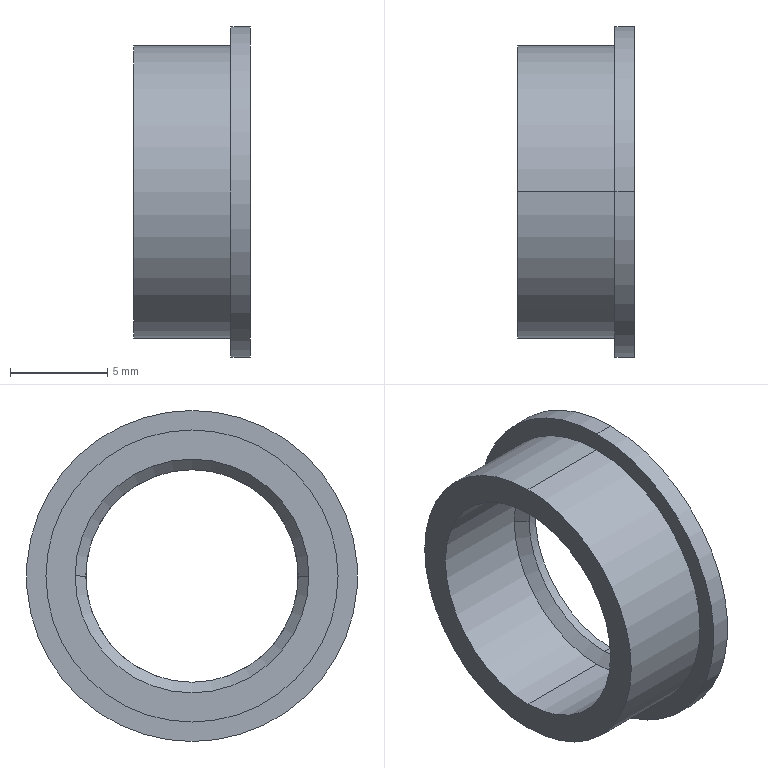Part | SolidWorks | features BaseBody 1 | 1 solid | 13 faces | box 6 x 17 x 17 mm | volume 446.259 mm3 | cylinder 8 | plane 3 | cone 2 | commonest cylinder face diameters 10.918 x2 12 x2 15 x2 17 x2
STEP:
#1=CARTESIAN_POINT('',(-6.5,0.,-7.5));
#2=VERTEX_POINT('',#1);
#3=CARTESIAN_POINT('',(-6.5,0.,7.5));
#4=VERTEX_POINT('',#3);
#5=CARTESIAN_POINT('',(-6.5,0.,0.));
#6=DIRECTION('',(1.,0.,0.));
#7=DIRECTION('',(0.,0.,-1.));
#8=AXIS2_PLACEMENT_3D('',#5,#6,#7);
#9=CIRCLE('',#8,7.5);
#10=EDGE_CURVE('',#2,#4,#9,.T.);
#11=ORIENTED_EDGE('',*,*,#10,.T.);
#12=CARTESIAN_POINT('',(-1.5,0.,7.5));
#13=VERTEX_POINT('',#12);
#14=CARTESIAN_POINT('',(-10.,0.,7.5));
#15=DIRECTION('',(1.,0.,0.));
#16=VECTOR('',#15,1000.);
#17=LINE('',#14,#16);
#18=EDGE_CURVE('',#4,#13,#17,.T.);
#19=ORIENTED_EDGE('',*,*,#18,.T.);
#20=CARTESIAN_POINT('',(-1.5,0.,-7.5));
#21=VERTEX_POINT('',#20);
#22=CARTESIAN_POINT('',(-1.5,0.,0.));
#23=DIRECTION('',(-1.,0.,0.));
#24=DIRECTION('',(0.,0.,-1.));
#25=AXIS2_PLACEMENT_3D('',#22,#23,#24);
#26=CIRCLE('',#25,7.5);
#27=EDGE_CURVE('',#13,#21,#26,.T.);
#28=ORIENTED_EDGE('',*,*,#27,.T.);
#29=CARTESIAN_POINT('',(-10.,0.,-7.5));
#30=DIRECTION('',(1.,0.,0.));
#31=VECTOR('',#30,1000.);
#32=LINE('',#29,#31);
#33=EDGE_CURVE('',#2,#21,#32,.T.);
#34=ORIENTED_EDGE('',*,*,#33,.F.);
#35=EDGE_LOOP('',(#11,#19,#28,#34));
#36=FACE_OUTER_BOUND('',#35,.T.);
#37=CARTESIAN_POINT('',(-10.,0.,0.));
#38=DIRECTION('',(1.,0.,0.));
#39=DIRECTION('',(0.,0.,-1.));
#40=AXIS2_PLACEMENT_3D('',#37,#38,#39);
#41=CYLINDRICAL_SURFACE('',#40,7.5);
#42=ADVANCED_FACE('',(#36),#41,.T.);
#43=CARTESIAN_POINT('',(-6.5,0.,6.));
#44=VERTEX_POINT('',#43);
#45=CARTESIAN_POINT('',(-6.5,0.,-6.));
#46=VERTEX_POINT('',#45);
#47=CARTESIAN_POINT('',(-6.5,0.,0.));
#48=DIRECTION('',(1.,0.,0.));
#49=DIRECTION('',(0.,0.,-1.));
#50=AXIS2_PLACEMENT_3D('',#47,#48,#49);
#51=CIRCLE('',#50,6.);
#52=EDGE_CURVE('',#44,#46,#51,.T.);
#53=ORIENTED_EDGE('',*,*,#52,.F.);
#54=CARTESIAN_POINT('',(-1.5,0.,6.));
#55=VERTEX_POINT('',#54);
#56=CARTESIAN_POINT('',(-10.,0.,6.));
#57=DIRECTION('',(1.,0.,0.));
#58=VECTOR('',#57,1000.);
#59=LINE('',#56,#58);
#60=EDGE_CURVE('',#44,#55,#59,.T.);
#61=ORIENTED_EDGE('',*,*,#60,.T.);
#62=CARTESIAN_POINT('',(-1.5,-6.,0.));
#63=VERTEX_POINT('',#62);
#64=CARTESIAN_POINT('',(-1.5,0.,0.));
#65=DIRECTION('',(-1.,0.,0.));
#66=DIRECTION('',(0.,0.,-1.));
#67=AXIS2_PLACEMENT_3D('',#64,#65,#66);
#68=CIRCLE('',#67,6.);
#69=EDGE_CURVE('',#63,#55,#68,.T.);
#70=ORIENTED_EDGE('',*,*,#69,.F.);
#71=CARTESIAN_POINT('',(-1.5,0.,-6.));
#72=VERTEX_POINT('',#71);
#73=CARTESIAN_POINT('',(-1.5,0.,0.));
#74=DIRECTION('',(-1.,0.,0.));
#75=DIRECTION('',(0.,0.,-1.));
#76=AXIS2_PLACEMENT_3D('',#73,#74,#75);
#77=CIRCLE('',#76,6.);
#78=EDGE_CURVE('',#72,#63,#77,.T.);
#79=ORIENTED_EDGE('',*,*,#78,.F.);
#80=CARTESIAN_POINT('',(-10.,0.,-6.));
#81=DIRECTION('',(1.,0.,0.));
#82=VECTOR('',#81,1000.);
#83=LINE('',#80,#82);
#84=EDGE_CURVE('',#46,#72,#83,.T.);
#85=ORIENTED_EDGE('',*,*,#84,.F.);
#86=EDGE_LOOP('',(#53,#61,#70,#79,#85));
#87=FACE_OUTER_BOUND('',#86,.T.);
#88=CARTESIAN_POINT('',(-10.,0.,0.));
#89=DIRECTION('',(1.,0.,0.));
#90=DIRECTION('',(0.,0.,-1.));
#91=AXIS2_PLACEMENT_3D('',#88,#89,#90);
#92=CYLINDRICAL_SURFACE('',#91,6.);
#93=ADVANCED_FACE('',(#87),#92,.F.);
#94=CARTESIAN_POINT('',(-1.5,0.,8.5));
#95=VERTEX_POINT('',#94);
#96=CARTESIAN_POINT('',(-1.5,0.,-8.5));
#97=VERTEX_POINT('',#96);
#98=CARTESIAN_POINT('',(-1.5,0.,0.));
#99=DIRECTION('',(-1.,0.,0.));
#100=DIRECTION('',(0.,0.,-1.));
#101=AXIS2_PLACEMENT_3D('',#98,#99,#100);
#102=CIRCLE('',#101,8.5);
#103=EDGE_CURVE('',#95,#97,#102,.T.);
#104=ORIENTED_EDGE('',*,*,#103,.F.);
#105=CARTESIAN_POINT('',(-0.5,0.,8.5));
#106=VERTEX_POINT('',#105);
#107=CARTESIAN_POINT('',(-10.,0.,8.5));
#108=DIRECTION('',(1.,0.,0.));
#109=VECTOR('',#108,1000.);
#110=LINE('',#107,#109);
#111=EDGE_CURVE('',#95,#106,#110,.T.);
#112=ORIENTED_EDGE('',*,*,#111,.T.);
#113=CARTESIAN_POINT('',(-0.5,0.,-8.5));
#114=VERTEX_POINT('',#113);
#115=CARTESIAN_POINT('',(-0.5,0.,0.));
#116=DIRECTION('',(-1.,0.,0.));
#117=DIRECTION('',(0.,0.,-1.));
#118=AXIS2_PLACEMENT_3D('',#115,#116,#117);
#119=CIRCLE('',#118,8.5);
#120=EDGE_CURVE('',#106,#114,#119,.T.);
#121=ORIENTED_EDGE('',*,*,#120,.T.);
#122=CARTESIAN_POINT('',(-10.,0.,-8.5));
#123=DIRECTION('',(1.,0.,0.));
#124=VECTOR('',#123,1000.);
#125=LINE('',#122,#124);
#126=EDGE_CURVE('',#97,#114,#125,.T.);
#127=ORIENTED_EDGE('',*,*,#126,.F.);
#128=EDGE_LOOP('',(#104,#112,#121,#127));
#129=FACE_OUTER_BOUND('',#128,.T.);
#130=CARTESIAN_POINT('',(-10.,0.,0.));
#131=DIRECTION('',(1.,0.,0.));
#132=DIRECTION('',(0.,0.,-1.));
#133=AXIS2_PLACEMENT_3D('',#130,#131,#132);
#134=CYLINDRICAL_SURFACE('',#133,8.5);
#135=ADVANCED_FACE('',(#129),#134,.T.);
#136=CARTESIAN_POINT('',(-0.959,5.459,0.));
#137=VERTEX_POINT('',#136);
#138=CARTESIAN_POINT('',(-0.959,0.,-5.459));
#139=VERTEX_POINT('',#138);
#140=CARTESIAN_POINT('',(-0.959,0.,0.));
#141=DIRECTION('',(-1.,0.,0.));
#142=DIRECTION('',(0.,0.,1.));
#143=AXIS2_PLACEMENT_3D('',#140,#141,#142);
#144=CIRCLE('',#143,5.459);
#145=EDGE_CURVE('',#137,#139,#144,.T.);
#146=ORIENTED_EDGE('',*,*,#145,.F.);
#147=CARTESIAN_POINT('',(-1.5,6.,0.));
#148=VERTEX_POINT('',#147);
#149=CARTESIAN_POINT('',(-1.5,6.,0.));
#150=DIRECTION('',(-0.7071,0.7071,0.));
#151=VECTOR('',#150,1000.);
#152=LINE('',#149,#151);
#153=EDGE_CURVE('',#137,#148,#152,.T.);
#154=ORIENTED_EDGE('',*,*,#153,.T.);
#155=CARTESIAN_POINT('',(-1.5,0.,0.));
#156=DIRECTION('',(-1.,0.,0.));
#157=DIRECTION('',(0.,0.,-1.));
#158=AXIS2_PLACEMENT_3D('',#155,#156,#157);
#159=CIRCLE('',#158,6.);
#160=EDGE_CURVE('',#148,#72,#159,.T.);
#161=ORIENTED_EDGE('',*,*,#160,.T.);
#162=ORIENTED_EDGE('',*,*,#78,.T.);
#163=CARTESIAN_POINT('',(-0.959,-5.459,0.));
#164=VERTEX_POINT('',#163);
#165=CARTESIAN_POINT('',(-1.5,-6.,0.));
#166=DIRECTION('',(-0.7071,-0.7071,0.));
#167=VECTOR('',#166,1000.);
#168=LINE('',#165,#167);
#169=EDGE_CURVE('',#164,#63,#168,.T.);
#170=ORIENTED_EDGE('',*,*,#169,.F.);
#171=CARTESIAN_POINT('',(-0.959,0.,0.));
#172=DIRECTION('',(-1.,0.,0.));
#173=DIRECTION('',(0.,0.,1.));
#174=AXIS2_PLACEMENT_3D('',#171,#172,#173);
#175=CIRCLE('',#174,5.459);
#176=EDGE_CURVE('',#139,#164,#175,.T.);
#177=ORIENTED_EDGE('',*,*,#176,.F.);
#178=EDGE_LOOP('',(#146,#154,#161,#162,#170,#177));
#179=FACE_OUTER_BOUND('',#178,.T.);
#180=CARTESIAN_POINT('',(-1.5,0.,0.));
#181=DIRECTION('',(-1.,0.,0.));
#182=DIRECTION('',(0.,-1.,0.));
#183=AXIS2_PLACEMENT_3D('',#180,#181,#182);
#184=CONICAL_SURFACE('',#183,6.,0.7854);
#185=ADVANCED_FACE('',(#179),#184,.F.);
#186=ORIENTED_EDGE('',*,*,#176,.T.);
#187=CARTESIAN_POINT('',(-0.959,0.,5.459));
#188=VERTEX_POINT('',#187);
#189=CARTESIAN_POINT('',(-0.959,0.,0.));
#190=DIRECTION('',(-1.,0.,0.));
#191=DIRECTION('',(0.,0.,1.));
#192=AXIS2_PLACEMENT_3D('',#189,#190,#191);
#193=CIRCLE('',#192,5.459);
#194=EDGE_CURVE('',#164,#188,#193,.T.);
#195=ORIENTED_EDGE('',*,*,#194,.T.);
#196=CARTESIAN_POINT('',(-0.5,0.,5.459));
#197=VERTEX_POINT('',#196);
#198=CARTESIAN_POINT('',(-10.,0.,5.459));
#199=DIRECTION('',(1.,0.,0.));
#200=VECTOR('',#199,1000.);
#201=LINE('',#198,#200);
#202=EDGE_CURVE('',#188,#197,#201,.T.);
#203=ORIENTED_EDGE('',*,*,#202,.T.);
#204=CARTESIAN_POINT('',(-0.5,0.,-5.459));
#205=VERTEX_POINT('',#204);
#206=CARTESIAN_POINT('',(-0.5,0.,0.));
#207=DIRECTION('',(-1.,0.,0.));
#208=DIRECTION('',(0.,0.,-1.));
#209=AXIS2_PLACEMENT_3D('',#206,#207,#208);
#210=CIRCLE('',#209,5.459);
#211=EDGE_CURVE('',#205,#197,#210,.T.);
#212=ORIENTED_EDGE('',*,*,#211,.F.);
#213=CARTESIAN_POINT('',(-10.,0.,-5.459));
#214=DIRECTION('',(1.,0.,0.));
#215=VECTOR('',#214,1000.);
#216=LINE('',#213,#215);
#217=EDGE_CURVE('',#139,#205,#216,.T.);
#218=ORIENTED_EDGE('',*,*,#217,.F.);
#219=EDGE_LOOP('',(#186,#195,#203,#212,#218));
#220=FACE_OUTER_BOUND('',#219,.T.);
#221=CARTESIAN_POINT('',(-10.,0.,0.));
#222=DIRECTION('',(1.,0.,0.));
#223=DIRECTION('',(0.,0.,-1.));
#224=AXIS2_PLACEMENT_3D('',#221,#222,#223);
#225=CYLINDRICAL_SURFACE('',#224,5.459);
#226=ADVANCED_FACE('',(#220),#225,.F.);
#227=ORIENTED_EDGE('',*,*,#18,.F.);
#228=CARTESIAN_POINT('',(-6.5,0.,0.));
#229=DIRECTION('',(1.,0.,0.));
#230=DIRECTION('',(0.,0.,-1.));
#231=AXIS2_PLACEMENT_3D('',#228,#229,#230);
#232=CIRCLE('',#231,7.5);
#233=EDGE_CURVE('',#4,#2,#232,.T.);
#234=ORIENTED_EDGE('',*,*,#233,.T.);
#235=ORIENTED_EDGE('',*,*,#33,.T.);
#236=CARTESIAN_POINT('',(-1.5,0.,0.));
#237=DIRECTION('',(-1.,0.,0.));
#238=DIRECTION('',(0.,0.,-1.));
#239=AXIS2_PLACEMENT_3D('',#236,#237,#238);
#240=CIRCLE('',#239,7.5);
#241=EDGE_CURVE('',#21,#13,#240,.T.);
#242=ORIENTED_EDGE('',*,*,#241,.T.);
#243=EDGE_LOOP('',(#227,#234,#235,#242));
#244=FACE_OUTER_BOUND('',#243,.T.);
#245=CARTESIAN_POINT('',(-10.,0.,0.));
#246=DIRECTION('',(1.,0.,0.));
#247=DIRECTION('',(0.,0.,-1.));
#248=AXIS2_PLACEMENT_3D('',#245,#246,#247);
#249=CYLINDRICAL_SURFACE('',#248,7.5);
#250=ADVANCED_FACE('',(#244),#249,.T.);
#251=CARTESIAN_POINT('',(-6.5,0.,0.));
#252=DIRECTION('',(1.,0.,0.));
#253=DIRECTION('',(0.,0.,-1.));
#254=AXIS2_PLACEMENT_3D('',#251,#252,#253);
#255=CIRCLE('',#254,6.);
#256=EDGE_CURVE('',#46,#44,#255,.T.);
#257=ORIENTED_EDGE('',*,*,#256,.T.);
#258=ORIENTED_EDGE('',*,*,#52,.T.);
#259=EDGE_LOOP('',(#257,#258));
#260=FACE_BOUND('',#259,.T.);
#261=ORIENTED_EDGE('',*,*,#10,.F.);
#262=ORIENTED_EDGE('',*,*,#233,.F.);
#263=EDGE_LOOP('',(#261,#262));
#264=FACE_OUTER_BOUND('',#263,.T.);
#265=CARTESIAN_POINT('',(-6.5,-6.,0.));
#266=DIRECTION('',(-1.,0.,0.));
#267=DIRECTION('',(0.,0.,1.));
#268=AXIS2_PLACEMENT_3D('',#265,#266,#267);
#269=PLANE('',#268);
#270=ADVANCED_FACE('',(#260,#264),#269,.T.);
#271=ORIENTED_EDGE('',*,*,#241,.F.);
#272=ORIENTED_EDGE('',*,*,#27,.F.);
#273=EDGE_LOOP('',(#271,#272));
#274=FACE_BOUND('',#273,.T.);
#275=CARTESIAN_POINT('',(-1.5,0.,0.));
#276=DIRECTION('',(-1.,0.,0.));
#277=DIRECTION('',(0.,0.,-1.));
#278=AXIS2_PLACEMENT_3D('',#275,#276,#277);
#279=CIRCLE('',#278,8.5);
#280=EDGE_CURVE('',#97,#95,#279,.T.);
#281=ORIENTED_EDGE('',*,*,#280,.T.);
#282=ORIENTED_EDGE('',*,*,#103,.T.);
#283=EDGE_LOOP('',(#281,#282));
#284=FACE_OUTER_BOUND('',#283,.T.);
#285=CARTESIAN_POINT('',(-1.5,-7.5,0.));
#286=DIRECTION('',(-1.,0.,0.));
#287=DIRECTION('',(0.,0.,1.));
#288=AXIS2_PLACEMENT_3D('',#285,#286,#287);
#289=PLANE('',#288);
#290=ADVANCED_FACE('',(#274,#284),#289,.T.);
#291=ORIENTED_EDGE('',*,*,#60,.F.);
#292=ORIENTED_EDGE('',*,*,#256,.F.);
#293=ORIENTED_EDGE('',*,*,#84,.T.);
#294=ORIENTED_EDGE('',*,*,#160,.F.);
#295=CARTESIAN_POINT('',(-1.5,0.,0.));
#296=DIRECTION('',(-1.,0.,0.));
#297=DIRECTION('',(0.,0.,-1.));
#298=AXIS2_PLACEMENT_3D('',#295,#296,#297);
#299=CIRCLE('',#298,6.);
#300=EDGE_CURVE('',#55,#148,#299,.T.);
#301=ORIENTED_EDGE('',*,*,#300,.F.);
#302=EDGE_LOOP('',(#291,#292,#293,#294,#301));
#303=FACE_OUTER_BOUND('',#302,.T.);
#304=CARTESIAN_POINT('',(-10.,0.,0.));
#305=DIRECTION('',(1.,0.,0.));
#306=DIRECTION('',(0.,0.,-1.));
#307=AXIS2_PLACEMENT_3D('',#304,#305,#306);
#308=CYLINDRICAL_SURFACE('',#307,6.);
#309=ADVANCED_FACE('',(#303),#308,.F.);
#310=ORIENTED_EDGE('',*,*,#111,.F.);
#311=ORIENTED_EDGE('',*,*,#280,.F.);
#312=ORIENTED_EDGE('',*,*,#126,.T.);
#313=CARTESIAN_POINT('',(-0.5,0.,0.));
#314=DIRECTION('',(-1.,0.,0.));
#315=DIRECTION('',(0.,0.,-1.));
#316=AXIS2_PLACEMENT_3D('',#313,#314,#315);
#317=CIRCLE('',#316,8.5);
#318=EDGE_CURVE('',#114,#106,#317,.T.);
#319=ORIENTED_EDGE('',*,*,#318,.T.);
#320=EDGE_LOOP('',(#310,#311,#312,#319));
#321=FACE_OUTER_BOUND('',#320,.T.);
#322=CARTESIAN_POINT('',(-10.,0.,0.));
#323=DIRECTION('',(1.,0.,0.));
#324=DIRECTION('',(0.,0.,-1.));
#325=AXIS2_PLACEMENT_3D('',#322,#323,#324);
#326=CYLINDRICAL_SURFACE('',#325,8.5);
#327=ADVANCED_FACE('',(#321),#326,.T.);
#328=ORIENTED_EDGE('',*,*,#153,.F.);
#329=CARTESIAN_POINT('',(-0.959,0.,0.));
#330=DIRECTION('',(-1.,0.,0.));
#331=DIRECTION('',(0.,0.,1.));
#332=AXIS2_PLACEMENT_3D('',#329,#330,#331);
#333=CIRCLE('',#332,5.459);
#334=EDGE_CURVE('',#188,#137,#333,.T.);
#335=ORIENTED_EDGE('',*,*,#334,.F.);
#336=ORIENTED_EDGE('',*,*,#194,.F.);
#337=ORIENTED_EDGE('',*,*,#169,.T.);
#338=ORIENTED_EDGE('',*,*,#69,.T.);
#339=ORIENTED_EDGE('',*,*,#300,.T.);
#340=EDGE_LOOP('',(#328,#335,#336,#337,#338,#339));
#341=FACE_OUTER_BOUND('',#340,.T.);
#342=CARTESIAN_POINT('',(-1.5,0.,0.));
#343=DIRECTION('',(-1.,0.,0.));
#344=DIRECTION('',(0.,-1.,0.));
#345=AXIS2_PLACEMENT_3D('',#342,#343,#344);
#346=CONICAL_SURFACE('',#345,6.,0.7854);
#347=ADVANCED_FACE('',(#341),#346,.F.);
#348=ORIENTED_EDGE('',*,*,#211,.T.);
#349=CARTESIAN_POINT('',(-0.5,0.,0.));
#350=DIRECTION('',(-1.,0.,0.));
#351=DIRECTION('',(0.,0.,-1.));
#352=AXIS2_PLACEMENT_3D('',#349,#350,#351);
#353=CIRCLE('',#352,5.459);
#354=EDGE_CURVE('',#197,#205,#353,.T.);
#355=ORIENTED_EDGE('',*,*,#354,.T.);
#356=EDGE_LOOP('',(#348,#355));
#357=FACE_BOUND('',#356,.T.);
#358=ORIENTED_EDGE('',*,*,#318,.F.);
#359=ORIENTED_EDGE('',*,*,#120,.F.);
#360=EDGE_LOOP('',(#358,#359));
#361=FACE_OUTER_BOUND('',#360,.T.);
#362=CARTESIAN_POINT('',(-0.5,0.,0.));
#363=DIRECTION('',(1.,0.,0.));
#364=DIRECTION('',(0.,0.,-1.));
#365=AXIS2_PLACEMENT_3D('',#362,#363,#364);
#366=PLANE('',#365);
#367=ADVANCED_FACE('',(#357,#361),#366,.T.);
#368=ORIENTED_EDGE('',*,*,#202,.F.);
#369=ORIENTED_EDGE('',*,*,#334,.T.);
#370=ORIENTED_EDGE('',*,*,#145,.T.);
#371=ORIENTED_EDGE('',*,*,#217,.T.);
#372=ORIENTED_EDGE('',*,*,#354,.F.);
#373=EDGE_LOOP('',(#368,#369,#370,#371,#372));
#374=FACE_OUTER_BOUND('',#373,.T.);
#375=CARTESIAN_POINT('',(-10.,0.,0.));
#376=DIRECTION('',(1.,0.,0.));
#377=DIRECTION('',(0.,0.,-1.));
#378=AXIS2_PLACEMENT_3D('',#375,#376,#377);
#379=CYLINDRICAL_SURFACE('',#378,5.459);
#380=ADVANCED_FACE('',(#374),#379,.F.);
#381=CLOSED_SHELL('',(#42,#93,#135,#185,#226,#250,#270,#290,#309,#327,#347,#367,#380));
#382=MANIFOLD_SOLID_BREP('',#381);
#383=CARTESIAN_POINT('',(0.,0.,0.));
#384=DIRECTION('',(0.,0.,1.));
#385=DIRECTION('',(1.,0.,0.));
#386=AXIS2_PLACEMENT_3D('',#383,#384,#385);
#387=(LENGTH_UNIT()NAMED_UNIT(*)SI_UNIT(.MILLI.,.METRE.));
#388=UNCERTAINTY_MEASURE_WITH_UNIT(LENGTH_MEASURE(0.00001),#387,'','');
#389=(NAMED_UNIT(*)PLANE_ANGLE_UNIT()SI_UNIT($,.RADIAN.));
#390=(NAMED_UNIT(*)SI_UNIT($,.STERADIAN.)SOLID_ANGLE_UNIT());
#391=(GEOMETRIC_REPRESENTATION_CONTEXT(3)GLOBAL_UNCERTAINTY_ASSIGNED_CONTEXT((#388))GLOBAL_UNIT_ASSIGNED_CONTEXT((#387,#389,#390))REPRESENTATION_CONTEXT('',''));
#392=ADVANCED_BREP_SHAPE_REPRESENTATION('',(#382,#386),#391);